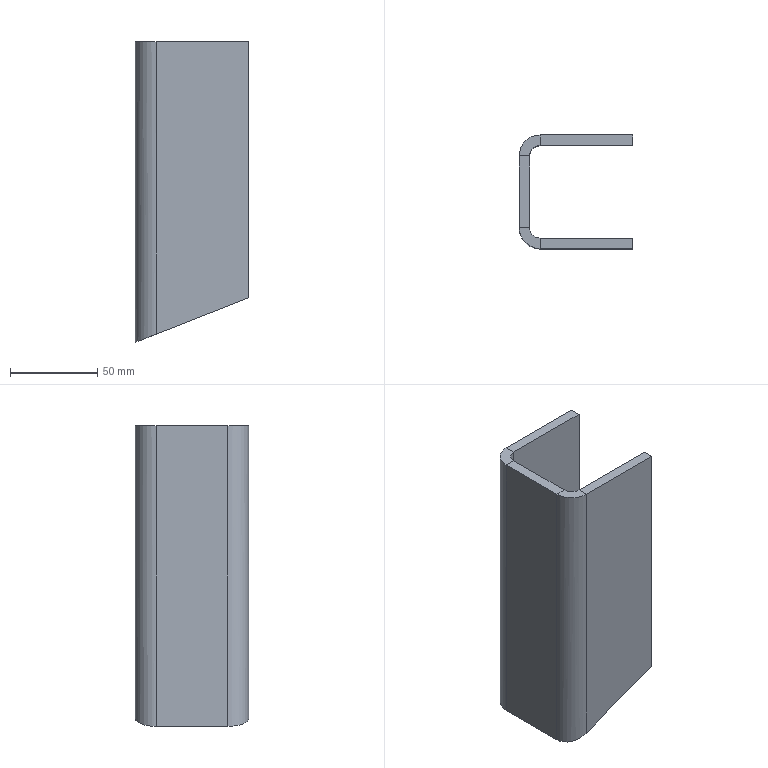Part | STEP file | 10-Bent plate | 1 solid | 18 faces | box 65 x 65 x 172 mm | volume 170584 mm3 | plane 14 | cylinder 4 | commonest cylinder face diameters 12 x2 24 x2
STEP:
#1=CARTESIAN_POINT('',(0.,0.,0.));
#2=DIRECTION('',(0.,0.,1.));
#3=DIRECTION('',(1.,0.,0.));
#4=AXIS2_PLACEMENT_3D('',#1,#2,#3);
#5=CARTESIAN_POINT('',(-53.,0.,172.));
#6=VERTEX_POINT('',#5);
#7=CARTESIAN_POINT('',(-53.,-6.,172.));
#8=VERTEX_POINT('',#7);
#9=CARTESIAN_POINT('',(-53.,0.,172.));
#10=DIRECTION('',(0.,-1.,0.));
#11=VECTOR('',#10,1.);
#12=LINE('',#9,#11);
#13=CARTESIAN_POINT('',(-53.,0.,172.));
#14=DIRECTION('',(0.,0.,1.));
#15=DIRECTION('',(1.,0.,0.));
#16=AXIS2_PLACEMENT_3D('',#13,#14,#15);
#17=PLANE('',#16);
#18=CARTESIAN_POINT('',(0.,0.));
#19=DIRECTION('',(0.,-1.));
#20=VECTOR('',#19,1.);
#21=LINE('',#18,#20);
#22=(GEOMETRIC_REPRESENTATION_CONTEXT(2)PARAMETRIC_REPRESENTATION_CONTEXT()REPRESENTATION_CONTEXT('',''));
#23=DEFINITIONAL_REPRESENTATION('',(#21),#22);
#24=PCURVE('',#17,#23);
#25=CARTESIAN_POINT('',(-59.,-12.,172.));
#26=DIRECTION('',(0.,0.,1.));
#27=DIRECTION('',(1.,0.,0.));
#28=AXIS2_PLACEMENT_3D('',#25,#26,#27);
#29=PLANE('',#28);
#30=CARTESIAN_POINT('',(6.,12.));
#31=DIRECTION('',(0.,-1.));
#32=VECTOR('',#31,1.);
#33=LINE('',#30,#32);
#34=(GEOMETRIC_REPRESENTATION_CONTEXT(2)PARAMETRIC_REPRESENTATION_CONTEXT()REPRESENTATION_CONTEXT('',''));
#35=DEFINITIONAL_REPRESENTATION('',(#33),#34);
#36=PCURVE('',#29,#35);
#37=SURFACE_CURVE('',#12,(#24,#36),.PCURVE_S1.);
#38=EDGE_CURVE('',#6,#8,#37,.T.);
#39=ORIENTED_EDGE('',*,*,#38,.F.);
#40=CARTESIAN_POINT('',(-65.,-12.,172.));
#41=VERTEX_POINT('',#40);
#42=CARTESIAN_POINT('',(-53.,-12.,172.));
#43=DIRECTION('',(0.,0.,1.));
#44=DIRECTION('',(-1.,0.,0.));
#45=AXIS2_PLACEMENT_3D('',#42,#43,#44);
#46=CIRCLE('',#45,12.);
#47=CARTESIAN_POINT('',(0.,-12.));
#48=DIRECTION('',(-1.,0.));
#49=AXIS2_PLACEMENT_2D('',#47,#48);
#50=CIRCLE('',#49,12.);
#51=(GEOMETRIC_REPRESENTATION_CONTEXT(2)PARAMETRIC_REPRESENTATION_CONTEXT()REPRESENTATION_CONTEXT('',''));
#52=DEFINITIONAL_REPRESENTATION('',(#50),#51);
#53=PCURVE('',#17,#52);
#54=CARTESIAN_POINT('',(-53.,-12.,172.));
#55=DIRECTION('',(0.,0.,-1.));
#56=DIRECTION('',(-1.,0.,0.));
#57=AXIS2_PLACEMENT_3D('',#54,#55,#56);
#58=CYLINDRICAL_SURFACE('',#57,12.);
#59=CARTESIAN_POINT('',(6.283,0.));
#60=DIRECTION('',(-1.,0.));
#61=VECTOR('',#60,1.);
#62=LINE('',#59,#61);
#63=(GEOMETRIC_REPRESENTATION_CONTEXT(2)PARAMETRIC_REPRESENTATION_CONTEXT()REPRESENTATION_CONTEXT('',''));
#64=DEFINITIONAL_REPRESENTATION('',(#62),#63);
#65=PCURVE('',#58,#64);
#66=SURFACE_CURVE('',#46,(#53,#65),.PCURVE_S1.);
#67=EDGE_CURVE('',#6,#41,#66,.T.);
#68=ORIENTED_EDGE('',*,*,#67,.T.);
#69=CARTESIAN_POINT('',(-59.,-12.,172.));
#70=VERTEX_POINT('',#69);
#71=CARTESIAN_POINT('',(-59.,-12.,172.));
#72=DIRECTION('',(-1.,0.,0.));
#73=VECTOR('',#72,1.);
#74=LINE('',#71,#73);
#75=CARTESIAN_POINT('',(-6.,-12.));
#76=DIRECTION('',(-1.,0.));
#77=VECTOR('',#76,1.);
#78=LINE('',#75,#77);
#79=(GEOMETRIC_REPRESENTATION_CONTEXT(2)PARAMETRIC_REPRESENTATION_CONTEXT()REPRESENTATION_CONTEXT('',''));
#80=DEFINITIONAL_REPRESENTATION('',(#78),#79);
#81=PCURVE('',#17,#80);
#82=CARTESIAN_POINT('',(-53.,-59.,172.));
#83=DIRECTION('',(0.,0.,1.));
#84=DIRECTION('',(1.,0.,0.));
#85=AXIS2_PLACEMENT_3D('',#82,#83,#84);
#86=PLANE('',#85);
#87=CARTESIAN_POINT('',(-6.,47.));
#88=DIRECTION('',(-1.,0.));
#89=VECTOR('',#88,1.);
#90=LINE('',#87,#89);
#91=(GEOMETRIC_REPRESENTATION_CONTEXT(2)PARAMETRIC_REPRESENTATION_CONTEXT()REPRESENTATION_CONTEXT('',''));
#92=DEFINITIONAL_REPRESENTATION('',(#90),#91);
#93=PCURVE('',#86,#92);
#94=SURFACE_CURVE('',#74,(#81,#93),.PCURVE_S1.);
#95=EDGE_CURVE('',#70,#41,#94,.T.);
#96=ORIENTED_EDGE('',*,*,#95,.F.);
#97=CARTESIAN_POINT('',(-53.,-12.,172.));
#98=DIRECTION('',(0.,0.,1.));
#99=DIRECTION('',(1.,0.,0.));
#100=AXIS2_PLACEMENT_3D('',#97,#98,#99);
#101=CIRCLE('',#100,6.);
#102=CARTESIAN_POINT('',(0.,-12.));
#103=DIRECTION('',(1.,0.));
#104=AXIS2_PLACEMENT_2D('',#102,#103);
#105=CIRCLE('',#104,6.);
#106=(GEOMETRIC_REPRESENTATION_CONTEXT(2)PARAMETRIC_REPRESENTATION_CONTEXT()REPRESENTATION_CONTEXT('',''));
#107=DEFINITIONAL_REPRESENTATION('',(#105),#106);
#108=PCURVE('',#17,#107);
#109=CARTESIAN_POINT('',(-53.,-12.,172.));
#110=DIRECTION('',(0.,0.,-1.));
#111=DIRECTION('',(-1.,0.,0.));
#112=AXIS2_PLACEMENT_3D('',#109,#110,#111);
#113=CYLINDRICAL_SURFACE('',#112,6.);
#114=CARTESIAN_POINT('',(3.142,0.));
#115=DIRECTION('',(-1.,0.));
#116=VECTOR('',#115,1.);
#117=LINE('',#114,#116);
#118=(GEOMETRIC_REPRESENTATION_CONTEXT(2)PARAMETRIC_REPRESENTATION_CONTEXT()REPRESENTATION_CONTEXT('',''));
#119=DEFINITIONAL_REPRESENTATION('',(#117),#118);
#120=PCURVE('',#113,#119);
#121=SURFACE_CURVE('',#101,(#108,#120),.PCURVE_S1.);
#122=EDGE_CURVE('',#8,#70,#121,.T.);
#123=ORIENTED_EDGE('',*,*,#122,.F.);
#124=EDGE_LOOP('',(#39,#68,#96,#123));
#125=FACE_BOUND('',#124,.T.);
#126=ADVANCED_FACE('',(#125),#17,.T.);
#127=CARTESIAN_POINT('',(0.,0.,172.));
#128=VERTEX_POINT('',#127);
#129=CARTESIAN_POINT('',(0.,0.,172.));
#130=DIRECTION('',(-1.,0.,0.));
#131=VECTOR('',#130,1.);
#132=LINE('',#129,#131);
#133=CARTESIAN_POINT('',(59.,12.));
#134=DIRECTION('',(-1.,0.));
#135=VECTOR('',#134,1.);
#136=LINE('',#133,#135);
#137=(GEOMETRIC_REPRESENTATION_CONTEXT(2)PARAMETRIC_REPRESENTATION_CONTEXT()REPRESENTATION_CONTEXT('',''));
#138=DEFINITIONAL_REPRESENTATION('',(#136),#137);
#139=PCURVE('',#29,#138);
#140=CARTESIAN_POINT('',(0.,0.,172.));
#141=DIRECTION('',(0.,-1.,0.));
#142=DIRECTION('',(1.,0.,0.));
#143=AXIS2_PLACEMENT_3D('',#140,#141,#142);
#144=PLANE('',#143);
#145=CARTESIAN_POINT('',(0.,0.));
#146=DIRECTION('',(-1.,0.));
#147=VECTOR('',#146,1.);
#148=LINE('',#145,#147);
#149=(GEOMETRIC_REPRESENTATION_CONTEXT(2)PARAMETRIC_REPRESENTATION_CONTEXT()REPRESENTATION_CONTEXT('',''));
#150=DEFINITIONAL_REPRESENTATION('',(#148),#149);
#151=PCURVE('',#144,#150);
#152=SURFACE_CURVE('',#132,(#139,#151),.PCURVE_S1.);
#153=EDGE_CURVE('',#128,#6,#152,.T.);
#154=ORIENTED_EDGE('',*,*,#153,.T.);
#155=ORIENTED_EDGE('',*,*,#38,.T.);
#156=CARTESIAN_POINT('',(0.,-6.,172.));
#157=VERTEX_POINT('',#156);
#158=CARTESIAN_POINT('',(0.,-6.,172.));
#159=DIRECTION('',(-1.,0.,0.));
#160=VECTOR('',#159,1.);
#161=LINE('',#158,#160);
#162=CARTESIAN_POINT('',(59.,6.));
#163=DIRECTION('',(-1.,0.));
#164=VECTOR('',#163,1.);
#165=LINE('',#162,#164);
#166=(GEOMETRIC_REPRESENTATION_CONTEXT(2)PARAMETRIC_REPRESENTATION_CONTEXT()REPRESENTATION_CONTEXT('',''));
#167=DEFINITIONAL_REPRESENTATION('',(#165),#166);
#168=PCURVE('',#29,#167);
#169=CARTESIAN_POINT('',(0.,-6.,172.));
#170=DIRECTION('',(0.,-1.,0.));
#171=DIRECTION('',(1.,0.,0.));
#172=AXIS2_PLACEMENT_3D('',#169,#170,#171);
#173=PLANE('',#172);
#174=CARTESIAN_POINT('',(0.,0.));
#175=DIRECTION('',(-1.,0.));
#176=VECTOR('',#175,1.);
#177=LINE('',#174,#176);
#178=(GEOMETRIC_REPRESENTATION_CONTEXT(2)PARAMETRIC_REPRESENTATION_CONTEXT()REPRESENTATION_CONTEXT('',''));
#179=DEFINITIONAL_REPRESENTATION('',(#177),#178);
#180=PCURVE('',#173,#179);
#181=SURFACE_CURVE('',#161,(#168,#180),.PCURVE_S1.);
#182=EDGE_CURVE('',#157,#8,#181,.T.);
#183=ORIENTED_EDGE('',*,*,#182,.F.);
#184=CARTESIAN_POINT('',(0.,0.,172.));
#185=DIRECTION('',(0.,-1.,0.));
#186=VECTOR('',#185,1.);
#187=LINE('',#184,#186);
#188=CARTESIAN_POINT('',(59.,12.));
#189=DIRECTION('',(0.,-1.));
#190=VECTOR('',#189,1.);
#191=LINE('',#188,#190);
#192=(GEOMETRIC_REPRESENTATION_CONTEXT(2)PARAMETRIC_REPRESENTATION_CONTEXT()REPRESENTATION_CONTEXT('',''));
#193=DEFINITIONAL_REPRESENTATION('',(#191),#192);
#194=PCURVE('',#29,#193);
#195=CARTESIAN_POINT('',(0.,0.,172.));
#196=DIRECTION('',(1.,0.,0.));
#197=DIRECTION('',(0.,1.,0.));
#198=AXIS2_PLACEMENT_3D('',#195,#196,#197);
#199=PLANE('',#198);
#200=CARTESIAN_POINT('',(0.,0.));
#201=DIRECTION('',(-1.,0.));
#202=VECTOR('',#201,1.);
#203=LINE('',#200,#202);
#204=(GEOMETRIC_REPRESENTATION_CONTEXT(2)PARAMETRIC_REPRESENTATION_CONTEXT()REPRESENTATION_CONTEXT('',''));
#205=DEFINITIONAL_REPRESENTATION('',(#203),#204);
#206=PCURVE('',#199,#205);
#207=SURFACE_CURVE('',#187,(#194,#206),.PCURVE_S1.);
#208=EDGE_CURVE('',#128,#157,#207,.T.);
#209=ORIENTED_EDGE('',*,*,#208,.F.);
#210=EDGE_LOOP('',(#154,#155,#183,#209));
#211=FACE_BOUND('',#210,.T.);
#212=ADVANCED_FACE('',(#211),#29,.T.);
#213=CARTESIAN_POINT('',(-65.,-53.,172.));
#214=VERTEX_POINT('',#213);
#215=CARTESIAN_POINT('',(-59.,-53.,172.));
#216=VERTEX_POINT('',#215);
#217=CARTESIAN_POINT('',(-65.,-53.,172.));
#218=DIRECTION('',(1.,0.,0.));
#219=VECTOR('',#218,1.);
#220=LINE('',#217,#219);
#221=CARTESIAN_POINT('',(-65.,-53.,172.));
#222=DIRECTION('',(0.,0.,1.));
#223=DIRECTION('',(1.,0.,0.));
#224=AXIS2_PLACEMENT_3D('',#221,#222,#223);
#225=PLANE('',#224);
#226=CARTESIAN_POINT('',(0.,0.));
#227=DIRECTION('',(1.,0.));
#228=VECTOR('',#227,1.);
#229=LINE('',#226,#228);
#230=(GEOMETRIC_REPRESENTATION_CONTEXT(2)PARAMETRIC_REPRESENTATION_CONTEXT()REPRESENTATION_CONTEXT('',''));
#231=DEFINITIONAL_REPRESENTATION('',(#229),#230);
#232=PCURVE('',#225,#231);
#233=CARTESIAN_POINT('',(-12.,6.));
#234=DIRECTION('',(1.,0.));
#235=VECTOR('',#234,1.);
#236=LINE('',#233,#235);
#237=(GEOMETRIC_REPRESENTATION_CONTEXT(2)PARAMETRIC_REPRESENTATION_CONTEXT()REPRESENTATION_CONTEXT('',''));
#238=DEFINITIONAL_REPRESENTATION('',(#236),#237);
#239=PCURVE('',#86,#238);
#240=SURFACE_CURVE('',#220,(#232,#239),.PCURVE_S1.);
#241=EDGE_CURVE('',#214,#216,#240,.T.);
#242=ORIENTED_EDGE('',*,*,#241,.F.);
#243=CARTESIAN_POINT('',(-53.,-65.,172.));
#244=VERTEX_POINT('',#243);
#245=CARTESIAN_POINT('',(-53.,-53.,172.));
#246=DIRECTION('',(0.,0.,1.));
#247=DIRECTION('',(-1.,0.,0.));
#248=AXIS2_PLACEMENT_3D('',#245,#246,#247);
#249=CIRCLE('',#248,12.);
#250=CARTESIAN_POINT('',(12.,0.));
#251=DIRECTION('',(-1.,0.));
#252=AXIS2_PLACEMENT_2D('',#250,#251);
#253=CIRCLE('',#252,12.);
#254=(GEOMETRIC_REPRESENTATION_CONTEXT(2)PARAMETRIC_REPRESENTATION_CONTEXT()REPRESENTATION_CONTEXT('',''));
#255=DEFINITIONAL_REPRESENTATION('',(#253),#254);
#256=PCURVE('',#225,#255);
#257=CARTESIAN_POINT('',(-53.,-53.,172.));
#258=DIRECTION('',(0.,0.,-1.));
#259=DIRECTION('',(-1.,0.,0.));
#260=AXIS2_PLACEMENT_3D('',#257,#258,#259);
#261=CYLINDRICAL_SURFACE('',#260,12.);
#262=CARTESIAN_POINT('',(6.283,0.));
#263=DIRECTION('',(-1.,0.));
#264=VECTOR('',#263,1.);
#265=LINE('',#262,#264);
#266=(GEOMETRIC_REPRESENTATION_CONTEXT(2)PARAMETRIC_REPRESENTATION_CONTEXT()REPRESENTATION_CONTEXT('',''));
#267=DEFINITIONAL_REPRESENTATION('',(#265),#266);
#268=PCURVE('',#261,#267);
#269=SURFACE_CURVE('',#249,(#256,#268),.PCURVE_S1.);
#270=EDGE_CURVE('',#214,#244,#269,.T.);
#271=ORIENTED_EDGE('',*,*,#270,.T.);
#272=CARTESIAN_POINT('',(-53.,-59.,172.));
#273=VERTEX_POINT('',#272);
#274=CARTESIAN_POINT('',(-53.,-59.,172.));
#275=DIRECTION('',(0.,-1.,0.));
#276=VECTOR('',#275,1.);
#277=LINE('',#274,#276);
#278=CARTESIAN_POINT('',(12.,-6.));
#279=DIRECTION('',(0.,-1.));
#280=VECTOR('',#279,1.);
#281=LINE('',#278,#280);
#282=(GEOMETRIC_REPRESENTATION_CONTEXT(2)PARAMETRIC_REPRESENTATION_CONTEXT()REPRESENTATION_CONTEXT('',''));
#283=DEFINITIONAL_REPRESENTATION('',(#281),#282);
#284=PCURVE('',#225,#283);
#285=CARTESIAN_POINT('',(-53.,-53.,172.));
#286=DIRECTION('',(0.,0.,1.));
#287=DIRECTION('',(1.,0.,0.));
#288=AXIS2_PLACEMENT_3D('',#285,#286,#287);
#289=PLANE('',#288);
#290=CARTESIAN_POINT('',(0.,-6.));
#291=DIRECTION('',(0.,-1.));
#292=VECTOR('',#291,1.);
#293=LINE('',#290,#292);
#294=(GEOMETRIC_REPRESENTATION_CONTEXT(2)PARAMETRIC_REPRESENTATION_CONTEXT()REPRESENTATION_CONTEXT('',''));
#295=DEFINITIONAL_REPRESENTATION('',(#293),#294);
#296=PCURVE('',#289,#295);
#297=SURFACE_CURVE('',#277,(#284,#296),.PCURVE_S1.);
#298=EDGE_CURVE('',#273,#244,#297,.T.);
#299=ORIENTED_EDGE('',*,*,#298,.F.);
#300=CARTESIAN_POINT('',(-53.,-53.,172.));
#301=DIRECTION('',(0.,0.,1.));
#302=DIRECTION('',(1.,0.,0.));
#303=AXIS2_PLACEMENT_3D('',#300,#301,#302);
#304=CIRCLE('',#303,6.);
#305=CARTESIAN_POINT('',(12.,0.));
#306=DIRECTION('',(1.,0.));
#307=AXIS2_PLACEMENT_2D('',#305,#306);
#308=CIRCLE('',#307,6.);
#309=(GEOMETRIC_REPRESENTATION_CONTEXT(2)PARAMETRIC_REPRESENTATION_CONTEXT()REPRESENTATION_CONTEXT('',''));
#310=DEFINITIONAL_REPRESENTATION('',(#308),#309);
#311=PCURVE('',#225,#310);
#312=CARTESIAN_POINT('',(-53.,-53.,172.));
#313=DIRECTION('',(0.,0.,-1.));
#314=DIRECTION('',(-1.,0.,0.));
#315=AXIS2_PLACEMENT_3D('',#312,#313,#314);
#316=CYLINDRICAL_SURFACE('',#315,6.);
#317=CARTESIAN_POINT('',(9.425,0.));
#318=DIRECTION('',(-1.,0.));
#319=VECTOR('',#318,1.);
#320=LINE('',#317,#319);
#321=(GEOMETRIC_REPRESENTATION_CONTEXT(2)PARAMETRIC_REPRESENTATION_CONTEXT()REPRESENTATION_CONTEXT('',''));
#322=DEFINITIONAL_REPRESENTATION('',(#320),#321);
#323=PCURVE('',#316,#322);
#324=SURFACE_CURVE('',#304,(#311,#323),.PCURVE_S1.);
#325=EDGE_CURVE('',#216,#273,#324,.T.);
#326=ORIENTED_EDGE('',*,*,#325,.F.);
#327=EDGE_LOOP('',(#242,#271,#299,#326));
#328=FACE_BOUND('',#327,.T.);
#329=ADVANCED_FACE('',(#328),#225,.T.);
#330=CARTESIAN_POINT('',(-65.,0.,172.));
#331=DIRECTION('',(0.,-1.,0.));
#332=VECTOR('',#331,1.);
#333=LINE('',#330,#332);
#334=CARTESIAN_POINT('',(-12.,59.));
#335=DIRECTION('',(0.,-1.));
#336=VECTOR('',#335,1.);
#337=LINE('',#334,#336);
#338=(GEOMETRIC_REPRESENTATION_CONTEXT(2)PARAMETRIC_REPRESENTATION_CONTEXT()REPRESENTATION_CONTEXT('',''));
#339=DEFINITIONAL_REPRESENTATION('',(#337),#338);
#340=PCURVE('',#86,#339);
#341=CARTESIAN_POINT('',(-65.,0.,172.));
#342=DIRECTION('',(1.,0.,0.));
#343=DIRECTION('',(0.,1.,0.));
#344=AXIS2_PLACEMENT_3D('',#341,#342,#343);
#345=PLANE('',#344);
#346=CARTESIAN_POINT('',(0.,0.));
#347=DIRECTION('',(-1.,0.));
#348=VECTOR('',#347,1.);
#349=LINE('',#346,#348);
#350=(GEOMETRIC_REPRESENTATION_CONTEXT(2)PARAMETRIC_REPRESENTATION_CONTEXT()REPRESENTATION_CONTEXT('',''));
#351=DEFINITIONAL_REPRESENTATION('',(#349),#350);
#352=PCURVE('',#345,#351);
#353=SURFACE_CURVE('',#333,(#340,#352),.PCURVE_S1.);
#354=EDGE_CURVE('',#41,#214,#353,.T.);
#355=ORIENTED_EDGE('',*,*,#354,.T.);
#356=ORIENTED_EDGE('',*,*,#241,.T.);
#357=CARTESIAN_POINT('',(-59.,0.,172.));
#358=DIRECTION('',(0.,-1.,0.));
#359=VECTOR('',#358,1.);
#360=LINE('',#357,#359);
#361=CARTESIAN_POINT('',(-6.,59.));
#362=DIRECTION('',(0.,-1.));
#363=VECTOR('',#362,1.);
#364=LINE('',#361,#363);
#365=(GEOMETRIC_REPRESENTATION_CONTEXT(2)PARAMETRIC_REPRESENTATION_CONTEXT()REPRESENTATION_CONTEXT('',''));
#366=DEFINITIONAL_REPRESENTATION('',(#364),#365);
#367=PCURVE('',#86,#366);
#368=CARTESIAN_POINT('',(-59.,0.,172.));
#369=DIRECTION('',(1.,0.,0.));
#370=DIRECTION('',(0.,1.,0.));
#371=AXIS2_PLACEMENT_3D('',#368,#369,#370);
#372=PLANE('',#371);
#373=CARTESIAN_POINT('',(0.,0.));
#374=DIRECTION('',(-1.,0.));
#375=VECTOR('',#374,1.);
#376=LINE('',#373,#375);
#377=(GEOMETRIC_REPRESENTATION_CONTEXT(2)PARAMETRIC_REPRESENTATION_CONTEXT()REPRESENTATION_CONTEXT('',''));
#378=DEFINITIONAL_REPRESENTATION('',(#376),#377);
#379=PCURVE('',#372,#378);
#380=SURFACE_CURVE('',#360,(#367,#379),.PCURVE_S1.);
#381=EDGE_CURVE('',#70,#216,#380,.T.);
#382=ORIENTED_EDGE('',*,*,#381,.F.);
#383=ORIENTED_EDGE('',*,*,#95,.T.);
#384=EDGE_LOOP('',(#355,#356,#382,#383));
#385=FACE_BOUND('',#384,.T.);
#386=ADVANCED_FACE('',(#385),#86,.T.);
#387=CARTESIAN_POINT('',(-53.,-65.,4.708));
#388=VERTEX_POINT('',#387);
#389=CARTESIAN_POINT('',(-53.,-65.,172.));
#390=DIRECTION('',(0.,0.,-1.));
#391=VECTOR('',#390,1.);
#392=LINE('',#389,#391);
#393=CARTESIAN_POINT('',(-65.,-65.,172.));
#394=DIRECTION('',(0.,1.,0.));
#395=DIRECTION('',(0.,0.,1.));
#396=AXIS2_PLACEMENT_3D('',#393,#394,#395);
#397=PLANE('',#396);
#398=CARTESIAN_POINT('',(0.,12.));
#399=DIRECTION('',(-1.,0.));
#400=VECTOR('',#399,1.);
#401=LINE('',#398,#400);
#402=(GEOMETRIC_REPRESENTATION_CONTEXT(2)PARAMETRIC_REPRESENTATION_CONTEXT()REPRESENTATION_CONTEXT('',''));
#403=DEFINITIONAL_REPRESENTATION('',(#401),#402);
#404=PCURVE('',#397,#403);
#405=CARTESIAN_POINT('',(4.712,0.));
#406=DIRECTION('',(0.,1.));
#407=VECTOR('',#406,1.);
#408=LINE('',#405,#407);
#409=(GEOMETRIC_REPRESENTATION_CONTEXT(2)PARAMETRIC_REPRESENTATION_CONTEXT()REPRESENTATION_CONTEXT('',''));
#410=DEFINITIONAL_REPRESENTATION('',(#408),#409);
#411=PCURVE('',#261,#410);
#412=SURFACE_CURVE('',#392,(#404,#411),.PCURVE_S1.);
#413=EDGE_CURVE('',#244,#388,#412,.T.);
#414=ORIENTED_EDGE('',*,*,#413,.T.);
#415=CARTESIAN_POINT('',(0.,-65.,25.5));
#416=VERTEX_POINT('',#415);
#417=CARTESIAN_POINT('',(-8.67,-65.,22.099));
#418=DIRECTION('',(0.9309,0.,0.3652));
#419=VECTOR('',#418,1.);
#420=LINE('',#417,#419);
#421=CARTESIAN_POINT('',(-149.901,56.33));
#422=DIRECTION('',(0.3652,0.9309));
#423=VECTOR('',#422,1.);
#424=LINE('',#421,#423);
#425=(GEOMETRIC_REPRESENTATION_CONTEXT(2)PARAMETRIC_REPRESENTATION_CONTEXT()REPRESENTATION_CONTEXT('',''));
#426=DEFINITIONAL_REPRESENTATION('',(#424),#425);
#427=PCURVE('',#397,#426);
#428=CARTESIAN_POINT('',(-8.67,-65.,22.099));
#429=DIRECTION('',(-0.3652,0.,0.9309));
#430=DIRECTION('',(0.9309,0.,0.3652));
#431=AXIS2_PLACEMENT_3D('',#428,#429,#430);
#432=PLANE('',#431);
#433=CARTESIAN_POINT('',(0.,0.));
#434=DIRECTION('',(1.,0.));
#435=VECTOR('',#434,1.);
#436=LINE('',#433,#435);
#437=(GEOMETRIC_REPRESENTATION_CONTEXT(2)PARAMETRIC_REPRESENTATION_CONTEXT()REPRESENTATION_CONTEXT('',''));
#438=DEFINITIONAL_REPRESENTATION('',(#436),#437);
#439=PCURVE('',#432,#438);
#440=SURFACE_CURVE('',#420,(#427,#439),.PCURVE_S1.);
#441=EDGE_CURVE('',#388,#416,#440,.T.);
#442=ORIENTED_EDGE('',*,*,#441,.T.);
#443=CARTESIAN_POINT('',(0.,-65.,172.));
#444=VERTEX_POINT('',#443);
#445=CARTESIAN_POINT('',(0.,-65.,172.));
#446=DIRECTION('',(0.,0.,-1.));
#447=VECTOR('',#446,1.);
#448=LINE('',#445,#447);
#449=CARTESIAN_POINT('',(0.,65.));
#450=DIRECTION('',(-1.,0.));
#451=VECTOR('',#450,1.);
#452=LINE('',#449,#451);
#453=(GEOMETRIC_REPRESENTATION_CONTEXT(2)PARAMETRIC_REPRESENTATION_CONTEXT()REPRESENTATION_CONTEXT('',''));
#454=DEFINITIONAL_REPRESENTATION('',(#452),#453);
#455=PCURVE('',#397,#454);
#456=CARTESIAN_POINT('',(0.,-59.,172.));
#457=DIRECTION('',(1.,0.,0.));
#458=DIRECTION('',(0.,0.,-1.));
#459=AXIS2_PLACEMENT_3D('',#456,#457,#458);
#460=PLANE('',#459);
#461=CARTESIAN_POINT('',(0.,-6.));
#462=DIRECTION('',(1.,0.));
#463=VECTOR('',#462,1.);
#464=LINE('',#461,#463);
#465=(GEOMETRIC_REPRESENTATION_CONTEXT(2)PARAMETRIC_REPRESENTATION_CONTEXT()REPRESENTATION_CONTEXT('',''));
#466=DEFINITIONAL_REPRESENTATION('',(#464),#465);
#467=PCURVE('',#460,#466);
#468=SURFACE_CURVE('',#448,(#455,#467),.PCURVE_S1.);
#469=EDGE_CURVE('',#444,#416,#468,.T.);
#470=ORIENTED_EDGE('',*,*,#469,.F.);
#471=CARTESIAN_POINT('',(-65.,-65.,172.));
#472=DIRECTION('',(1.,0.,0.));
#473=VECTOR('',#472,1.);
#474=LINE('',#471,#473);
#475=CARTESIAN_POINT('',(0.,0.));
#476=DIRECTION('',(0.,1.));
#477=VECTOR('',#476,1.);
#478=LINE('',#475,#477);
#479=(GEOMETRIC_REPRESENTATION_CONTEXT(2)PARAMETRIC_REPRESENTATION_CONTEXT()REPRESENTATION_CONTEXT('',''));
#480=DEFINITIONAL_REPRESENTATION('',(#478),#479);
#481=PCURVE('',#397,#480);
#482=CARTESIAN_POINT('',(-12.,-12.));
#483=DIRECTION('',(1.,0.));
#484=VECTOR('',#483,1.);
#485=LINE('',#482,#484);
#486=(GEOMETRIC_REPRESENTATION_CONTEXT(2)PARAMETRIC_REPRESENTATION_CONTEXT()REPRESENTATION_CONTEXT('',''));
#487=DEFINITIONAL_REPRESENTATION('',(#485),#486);
#488=PCURVE('',#289,#487);
#489=SURFACE_CURVE('',#474,(#481,#488),.PCURVE_S1.);
#490=EDGE_CURVE('',#244,#444,#489,.T.);
#491=ORIENTED_EDGE('',*,*,#490,.F.);
#492=EDGE_LOOP('',(#414,#442,#470,#491));
#493=FACE_BOUND('',#492,.T.);
#494=ADVANCED_FACE('',(#493),#397,.F.);
#495=CARTESIAN_POINT('',(0.,-59.,25.5));
#496=VERTEX_POINT('',#495);
#497=CARTESIAN_POINT('',(0.,-65.,25.5));
#498=DIRECTION('',(0.,1.,0.));
#499=VECTOR('',#498,1.);
#500=LINE('',#497,#499);
#501=CARTESIAN_POINT('',(146.5,-6.));
#502=DIRECTION('',(0.,1.));
#503=VECTOR('',#502,1.);
#504=LINE('',#501,#503);
#505=(GEOMETRIC_REPRESENTATION_CONTEXT(2)PARAMETRIC_REPRESENTATION_CONTEXT()REPRESENTATION_CONTEXT('',''));
#506=DEFINITIONAL_REPRESENTATION('',(#504),#505);
#507=PCURVE('',#460,#506);
#508=CARTESIAN_POINT('',(9.313,0.));
#509=DIRECTION('',(0.,1.));
#510=VECTOR('',#509,1.);
#511=LINE('',#508,#510);
#512=(GEOMETRIC_REPRESENTATION_CONTEXT(2)PARAMETRIC_REPRESENTATION_CONTEXT()REPRESENTATION_CONTEXT('',''));
#513=DEFINITIONAL_REPRESENTATION('',(#511),#512);
#514=PCURVE('',#432,#513);
#515=SURFACE_CURVE('',#500,(#507,#514),.PCURVE_S1.);
#516=EDGE_CURVE('',#416,#496,#515,.T.);
#517=ORIENTED_EDGE('',*,*,#516,.T.);
#518=CARTESIAN_POINT('',(0.,-59.,172.));
#519=VERTEX_POINT('',#518);
#520=CARTESIAN_POINT('',(0.,-59.,172.));
#521=DIRECTION('',(0.,0.,-1.));
#522=VECTOR('',#521,1.);
#523=LINE('',#520,#522);
#524=CARTESIAN_POINT('',(0.,0.));
#525=DIRECTION('',(1.,0.));
#526=VECTOR('',#525,1.);
#527=LINE('',#524,#526);
#528=(GEOMETRIC_REPRESENTATION_CONTEXT(2)PARAMETRIC_REPRESENTATION_CONTEXT()REPRESENTATION_CONTEXT('',''));
#529=DEFINITIONAL_REPRESENTATION('',(#527),#528);
#530=PCURVE('',#460,#529);
#531=CARTESIAN_POINT('',(-65.,-59.,172.));
#532=DIRECTION('',(0.,1.,0.));
#533=DIRECTION('',(0.,0.,1.));
#534=AXIS2_PLACEMENT_3D('',#531,#532,#533);
#535=PLANE('',#534);
#536=CARTESIAN_POINT('',(0.,65.));
#537=DIRECTION('',(-1.,0.));
#538=VECTOR('',#537,1.);
#539=LINE('',#536,#538);
#540=(GEOMETRIC_REPRESENTATION_CONTEXT(2)PARAMETRIC_REPRESENTATION_CONTEXT()REPRESENTATION_CONTEXT('',''));
#541=DEFINITIONAL_REPRESENTATION('',(#539),#540);
#542=PCURVE('',#535,#541);
#543=SURFACE_CURVE('',#523,(#530,#542),.PCURVE_S1.);
#544=EDGE_CURVE('',#519,#496,#543,.T.);
#545=ORIENTED_EDGE('',*,*,#544,.F.);
#546=CARTESIAN_POINT('',(0.,-59.,172.));
#547=DIRECTION('',(0.,-1.,0.));
#548=VECTOR('',#547,1.);
#549=LINE('',#546,#548);
#550=CARTESIAN_POINT('',(0.,0.));
#551=DIRECTION('',(0.,-1.));
#552=VECTOR('',#551,1.);
#553=LINE('',#550,#552);
#554=(GEOMETRIC_REPRESENTATION_CONTEXT(2)PARAMETRIC_REPRESENTATION_CONTEXT()REPRESENTATION_CONTEXT('',''));
#555=DEFINITIONAL_REPRESENTATION('',(#553),#554);
#556=PCURVE('',#460,#555);
#557=CARTESIAN_POINT('',(53.,-6.));
#558=DIRECTION('',(0.,-1.));
#559=VECTOR('',#558,1.);
#560=LINE('',#557,#559);
#561=(GEOMETRIC_REPRESENTATION_CONTEXT(2)PARAMETRIC_REPRESENTATION_CONTEXT()REPRESENTATION_CONTEXT('',''));
#562=DEFINITIONAL_REPRESENTATION('',(#560),#561);
#563=PCURVE('',#289,#562);
#564=SURFACE_CURVE('',#549,(#556,#563),.PCURVE_S1.);
#565=EDGE_CURVE('',#519,#444,#564,.T.);
#566=ORIENTED_EDGE('',*,*,#565,.T.);
#567=ORIENTED_EDGE('',*,*,#469,.T.);
#568=EDGE_LOOP('',(#517,#545,#566,#567));
#569=FACE_BOUND('',#568,.T.);
#570=ADVANCED_FACE('',(#569),#460,.T.);
#571=CARTESIAN_POINT('',(-53.,-59.,4.708));
#572=VERTEX_POINT('',#571);
#573=CARTESIAN_POINT('',(-6.523,-59.,22.941));
#574=DIRECTION('',(0.9309,0.,0.3652));
#575=VECTOR('',#574,1.);
#576=LINE('',#573,#575);
#577=CARTESIAN_POINT('',(-149.059,58.477));
#578=DIRECTION('',(0.3652,0.9309));
#579=VECTOR('',#578,1.);
#580=LINE('',#577,#579);
#581=(GEOMETRIC_REPRESENTATION_CONTEXT(2)PARAMETRIC_REPRESENTATION_CONTEXT()REPRESENTATION_CONTEXT('',''));
#582=DEFINITIONAL_REPRESENTATION('',(#580),#581);
#583=PCURVE('',#535,#582);
#584=CARTESIAN_POINT('',(2.306,6.));
#585=DIRECTION('',(1.,0.));
#586=VECTOR('',#585,1.);
#587=LINE('',#584,#586);
#588=(GEOMETRIC_REPRESENTATION_CONTEXT(2)PARAMETRIC_REPRESENTATION_CONTEXT()REPRESENTATION_CONTEXT('',''));
#589=DEFINITIONAL_REPRESENTATION('',(#587),#588);
#590=PCURVE('',#432,#589);
#591=SURFACE_CURVE('',#576,(#583,#590),.PCURVE_S1.);
#592=EDGE_CURVE('',#572,#496,#591,.T.);
#593=ORIENTED_EDGE('',*,*,#592,.F.);
#594=CARTESIAN_POINT('',(-53.,-59.,172.));
#595=DIRECTION('',(0.,0.,-1.));
#596=VECTOR('',#595,1.);
#597=LINE('',#594,#596);
#598=CARTESIAN_POINT('',(0.,12.));
#599=DIRECTION('',(-1.,0.));
#600=VECTOR('',#599,1.);
#601=LINE('',#598,#600);
#602=(GEOMETRIC_REPRESENTATION_CONTEXT(2)PARAMETRIC_REPRESENTATION_CONTEXT()REPRESENTATION_CONTEXT('',''));
#603=DEFINITIONAL_REPRESENTATION('',(#601),#602);
#604=PCURVE('',#535,#603);
#605=CARTESIAN_POINT('',(4.712,0.));
#606=DIRECTION('',(0.,1.));
#607=VECTOR('',#606,1.);
#608=LINE('',#605,#607);
#609=(GEOMETRIC_REPRESENTATION_CONTEXT(2)PARAMETRIC_REPRESENTATION_CONTEXT()REPRESENTATION_CONTEXT('',''));
#610=DEFINITIONAL_REPRESENTATION('',(#608),#609);
#611=PCURVE('',#316,#610);
#612=SURFACE_CURVE('',#597,(#604,#611),.PCURVE_S1.);
#613=EDGE_CURVE('',#273,#572,#612,.T.);
#614=ORIENTED_EDGE('',*,*,#613,.F.);
#615=CARTESIAN_POINT('',(-65.,-59.,172.));
#616=DIRECTION('',(1.,0.,0.));
#617=VECTOR('',#616,1.);
#618=LINE('',#615,#617);
#619=CARTESIAN_POINT('',(0.,0.));
#620=DIRECTION('',(0.,1.));
#621=VECTOR('',#620,1.);
#622=LINE('',#619,#621);
#623=(GEOMETRIC_REPRESENTATION_CONTEXT(2)PARAMETRIC_REPRESENTATION_CONTEXT()REPRESENTATION_CONTEXT('',''));
#624=DEFINITIONAL_REPRESENTATION('',(#622),#623);
#625=PCURVE('',#535,#624);
#626=CARTESIAN_POINT('',(-12.,-6.));
#627=DIRECTION('',(1.,0.));
#628=VECTOR('',#627,1.);
#629=LINE('',#626,#628);
#630=(GEOMETRIC_REPRESENTATION_CONTEXT(2)PARAMETRIC_REPRESENTATION_CONTEXT()REPRESENTATION_CONTEXT('',''));
#631=DEFINITIONAL_REPRESENTATION('',(#629),#630);
#632=PCURVE('',#289,#631);
#633=SURFACE_CURVE('',#618,(#625,#632),.PCURVE_S1.);
#634=EDGE_CURVE('',#273,#519,#633,.T.);
#635=ORIENTED_EDGE('',*,*,#634,.T.);
#636=ORIENTED_EDGE('',*,*,#544,.T.);
#637=EDGE_LOOP('',(#593,#614,#635,#636));
#638=FACE_BOUND('',#637,.T.);
#639=ADVANCED_FACE('',(#638),#535,.T.);
#640=ORIENTED_EDGE('',*,*,#613,.F.);
#641=ORIENTED_EDGE('',*,*,#325,.F.);
#642=CARTESIAN_POINT('',(-59.,-53.,2.354));
#643=VERTEX_POINT('',#642);
#644=CARTESIAN_POINT('',(-59.,-53.,172.));
#645=DIRECTION('',(0.,0.,-1.));
#646=VECTOR('',#645,1.);
#647=LINE('',#644,#646);
#648=CARTESIAN_POINT('',(6.283,0.));
#649=DIRECTION('',(0.,1.));
#650=VECTOR('',#649,1.);
#651=LINE('',#648,#650);
#652=(GEOMETRIC_REPRESENTATION_CONTEXT(2)PARAMETRIC_REPRESENTATION_CONTEXT()REPRESENTATION_CONTEXT('',''));
#653=DEFINITIONAL_REPRESENTATION('',(#651),#652);
#654=PCURVE('',#316,#653);
#655=CARTESIAN_POINT('',(-53.,0.));
#656=DIRECTION('',(0.,-1.));
#657=VECTOR('',#656,1.);
#658=LINE('',#655,#657);
#659=(GEOMETRIC_REPRESENTATION_CONTEXT(2)PARAMETRIC_REPRESENTATION_CONTEXT()REPRESENTATION_CONTEXT('',''));
#660=DEFINITIONAL_REPRESENTATION('',(#658),#659);
#661=PCURVE('',#372,#660);
#662=SURFACE_CURVE('',#647,(#654,#661),.PCURVE_S1.);
#663=EDGE_CURVE('',#216,#643,#662,.T.);
#664=ORIENTED_EDGE('',*,*,#663,.T.);
#665=CARTESIAN_POINT('',(-59.,-53.,2.354));
#666=CARTESIAN_POINT('',(-59.,-56.515,2.354));
#667=CARTESIAN_POINT('',(-56.515,-59.,3.329));
#668=CARTESIAN_POINT('',(-53.,-59.,4.708));
#669=(BOUNDED_CURVE()B_SPLINE_CURVE(3,(#665,#666,#667,#668),.UNSPECIFIED.,.F.,.F.)B_SPLINE_CURVE_WITH_KNOTS((4,4),(0.,1.571),.PIECEWISE_BEZIER_KNOTS.)CURVE()GEOMETRIC_REPRESENTATION_ITEM()RATIONAL_B_SPLINE_CURVE((1.,0.8047,0.8047,1.))REPRESENTATION_ITEM(''));
#670=CARTESIAN_POINT('',(6.283,169.646));
#671=CARTESIAN_POINT('',(6.262,169.646));
#672=CARTESIAN_POINT('',(6.218,169.643));
#673=CARTESIAN_POINT('',(6.152,169.628));
#674=CARTESIAN_POINT('',(6.083,169.601));
#675=CARTESIAN_POINT('',(6.013,169.563));
#676=CARTESIAN_POINT('',(5.942,169.513));
#677=CARTESIAN_POINT('',(5.87,169.45));
#678=CARTESIAN_POINT('',(5.797,169.375));
#679=CARTESIAN_POINT('',(5.723,169.288));
#680=CARTESIAN_POINT('',(5.648,169.189));
#681=CARTESIAN_POINT('',(5.573,169.079));
#682=CARTESIAN_POINT('',(5.498,168.958));
#683=CARTESIAN_POINT('',(5.422,168.828));
#684=CARTESIAN_POINT('',(5.347,168.69));
#685=CARTESIAN_POINT('',(5.273,168.544));
#686=CARTESIAN_POINT('',(5.199,168.393));
#687=CARTESIAN_POINT('',(5.125,168.238));
#688=CARTESIAN_POINT('',(5.053,168.08));
#689=CARTESIAN_POINT('',(4.982,167.92));
#690=CARTESIAN_POINT('',(4.912,167.76));
#691=CARTESIAN_POINT('',(4.844,167.601));
#692=CARTESIAN_POINT('',(4.777,167.445));
#693=CARTESIAN_POINT('',(4.734,167.343));
#694=CARTESIAN_POINT('',(4.712,167.292));
#695=B_SPLINE_CURVE_WITH_KNOTS('',3,(#670,#671,#672,#673,#674,#675,#676,#677,#678,#679,#680,#681,#682,#683,#684,#685,#686,#687,#688,#689,#690,#691,#692,#693,#694),.UNSPECIFIED.,.F.,.F.,(4,1,1,1,1,1,1,1,1,1,1,1,1,1,1,1,1,1,1,1,1,1,4),(0.,0.0714,0.1428,0.2142,0.2856,0.357,0.4284,0.4998,0.5712,0.6426,0.714,0.7854,0.8568,0.9282,0.9996,1.071,1.142,1.214,1.285,1.357,1.428,1.499,1.571),.QUASI_UNIFORM_KNOTS.);
#696=(GEOMETRIC_REPRESENTATION_CONTEXT(2)PARAMETRIC_REPRESENTATION_CONTEXT()REPRESENTATION_CONTEXT('',''));
#697=DEFINITIONAL_REPRESENTATION('',(#695),#696);
#698=PCURVE('',#316,#697);
#699=CARTESIAN_POINT('',(-54.065,12.));
#700=CARTESIAN_POINT('',(-54.065,8.485));
#701=CARTESIAN_POINT('',(-51.395,6.));
#702=CARTESIAN_POINT('',(-47.62,6.));
#703=(BOUNDED_CURVE()B_SPLINE_CURVE(3,(#699,#700,#701,#702),.UNSPECIFIED.,.F.,.F.)B_SPLINE_CURVE_WITH_KNOTS((4,4),(0.,1.571),.PIECEWISE_BEZIER_KNOTS.)CURVE()GEOMETRIC_REPRESENTATION_ITEM()RATIONAL_B_SPLINE_CURVE((1.,0.8047,0.8047,1.))REPRESENTATION_ITEM(''));
#704=(GEOMETRIC_REPRESENTATION_CONTEXT(2)PARAMETRIC_REPRESENTATION_CONTEXT()REPRESENTATION_CONTEXT('',''));
#705=DEFINITIONAL_REPRESENTATION('',(#703),#704);
#706=PCURVE('',#432,#705);
#707=SURFACE_CURVE('',#669,(#698,#706),.PCURVE_S1.);
#708=EDGE_CURVE('',#643,#572,#707,.T.);
#709=ORIENTED_EDGE('',*,*,#708,.T.);
#710=EDGE_LOOP('',(#640,#641,#664,#709));
#711=FACE_BOUND('',#710,.F.);
#712=ADVANCED_FACE('',(#711),#316,.F.);
#713=CARTESIAN_POINT('',(-59.,-12.,2.354));
#714=VERTEX_POINT('',#713);
#715=CARTESIAN_POINT('',(-59.,0.,2.354));
#716=DIRECTION('',(0.,-1.,0.));
#717=VECTOR('',#716,1.);
#718=LINE('',#715,#717);
#719=CARTESIAN_POINT('',(0.,-169.646));
#720=DIRECTION('',(-1.,0.));
#721=VECTOR('',#720,1.);
#722=LINE('',#719,#721);
#723=(GEOMETRIC_REPRESENTATION_CONTEXT(2)PARAMETRIC_REPRESENTATION_CONTEXT()REPRESENTATION_CONTEXT('',''));
#724=DEFINITIONAL_REPRESENTATION('',(#722),#723);
#725=PCURVE('',#372,#724);
#726=CARTESIAN_POINT('',(-54.065,65.));
#727=DIRECTION('',(0.,-1.));
#728=VECTOR('',#727,1.);
#729=LINE('',#726,#728);
#730=(GEOMETRIC_REPRESENTATION_CONTEXT(2)PARAMETRIC_REPRESENTATION_CONTEXT()REPRESENTATION_CONTEXT('',''));
#731=DEFINITIONAL_REPRESENTATION('',(#729),#730);
#732=PCURVE('',#432,#731);
#733=SURFACE_CURVE('',#718,(#725,#732),.PCURVE_S1.);
#734=EDGE_CURVE('',#714,#643,#733,.T.);
#735=ORIENTED_EDGE('',*,*,#734,.F.);
#736=CARTESIAN_POINT('',(-59.,-12.,172.));
#737=DIRECTION('',(0.,0.,-1.));
#738=VECTOR('',#737,1.);
#739=LINE('',#736,#738);
#740=CARTESIAN_POINT('',(-12.,0.));
#741=DIRECTION('',(0.,-1.));
#742=VECTOR('',#741,1.);
#743=LINE('',#740,#742);
#744=(GEOMETRIC_REPRESENTATION_CONTEXT(2)PARAMETRIC_REPRESENTATION_CONTEXT()REPRESENTATION_CONTEXT('',''));
#745=DEFINITIONAL_REPRESENTATION('',(#743),#744);
#746=PCURVE('',#372,#745);
#747=CARTESIAN_POINT('',(0.,0.));
#748=DIRECTION('',(0.,1.));
#749=VECTOR('',#748,1.);
#750=LINE('',#747,#749);
#751=(GEOMETRIC_REPRESENTATION_CONTEXT(2)PARAMETRIC_REPRESENTATION_CONTEXT()REPRESENTATION_CONTEXT('',''));
#752=DEFINITIONAL_REPRESENTATION('',(#750),#751);
#753=PCURVE('',#113,#752);
#754=SURFACE_CURVE('',#739,(#746,#753),.PCURVE_S1.);
#755=EDGE_CURVE('',#70,#714,#754,.T.);
#756=ORIENTED_EDGE('',*,*,#755,.F.);
#757=ORIENTED_EDGE('',*,*,#381,.T.);
#758=ORIENTED_EDGE('',*,*,#663,.T.);
#759=EDGE_LOOP('',(#735,#756,#757,#758));
#760=FACE_BOUND('',#759,.T.);
#761=ADVANCED_FACE('',(#760),#372,.T.);
#762=ORIENTED_EDGE('',*,*,#755,.F.);
#763=ORIENTED_EDGE('',*,*,#122,.F.);
#764=CARTESIAN_POINT('',(-53.,-6.,4.708));
#765=VERTEX_POINT('',#764);
#766=CARTESIAN_POINT('',(-53.,-6.,172.));
#767=DIRECTION('',(0.,0.,-1.));
#768=VECTOR('',#767,1.);
#769=LINE('',#766,#768);
#770=CARTESIAN_POINT('',(1.571,0.));
#771=DIRECTION('',(0.,1.));
#772=VECTOR('',#771,1.);
#773=LINE('',#770,#772);
#774=(GEOMETRIC_REPRESENTATION_CONTEXT(2)PARAMETRIC_REPRESENTATION_CONTEXT()REPRESENTATION_CONTEXT('',''));
#775=DEFINITIONAL_REPRESENTATION('',(#773),#774);
#776=PCURVE('',#113,#775);
#777=CARTESIAN_POINT('',(-53.,0.));
#778=DIRECTION('',(0.,-1.));
#779=VECTOR('',#778,1.);
#780=LINE('',#777,#779);
#781=(GEOMETRIC_REPRESENTATION_CONTEXT(2)PARAMETRIC_REPRESENTATION_CONTEXT()REPRESENTATION_CONTEXT('',''));
#782=DEFINITIONAL_REPRESENTATION('',(#780),#781);
#783=PCURVE('',#173,#782);
#784=SURFACE_CURVE('',#769,(#776,#783),.PCURVE_S1.);
#785=EDGE_CURVE('',#8,#765,#784,.T.);
#786=ORIENTED_EDGE('',*,*,#785,.T.);
#787=CARTESIAN_POINT('',(-53.,-6.,4.708));
#788=CARTESIAN_POINT('',(-56.515,-6.,3.329));
#789=CARTESIAN_POINT('',(-59.,-8.485,2.354));
#790=CARTESIAN_POINT('',(-59.,-12.,2.354));
#791=(BOUNDED_CURVE()B_SPLINE_CURVE(3,(#787,#788,#789,#790),.UNSPECIFIED.,.F.,.F.)B_SPLINE_CURVE_WITH_KNOTS((4,4),(4.712,6.283),.PIECEWISE_BEZIER_KNOTS.)CURVE()GEOMETRIC_REPRESENTATION_ITEM()RATIONAL_B_SPLINE_CURVE((1.,0.8047,0.8047,1.))REPRESENTATION_ITEM(''));
#792=CARTESIAN_POINT('',(1.571,167.292));
#793=CARTESIAN_POINT('',(1.549,167.343));
#794=CARTESIAN_POINT('',(1.506,167.445));
#795=CARTESIAN_POINT('',(1.439,167.601));
#796=CARTESIAN_POINT('',(1.371,167.76));
#797=CARTESIAN_POINT('',(1.301,167.92));
#798=CARTESIAN_POINT('',(1.23,168.08));
#799=CARTESIAN_POINT('',(1.158,168.238));
#800=CARTESIAN_POINT('',(1.085,168.393));
#801=CARTESIAN_POINT('',(1.01,168.544));
#802=CARTESIAN_POINT('',(0.9358,168.69));
#803=CARTESIAN_POINT('',(0.8607,168.828));
#804=CARTESIAN_POINT('',(0.7854,168.958));
#805=CARTESIAN_POINT('',(0.7101,169.079));
#806=CARTESIAN_POINT('',(0.635,169.189));
#807=CARTESIAN_POINT('',(0.5603,169.288));
#808=CARTESIAN_POINT('',(0.4863,169.375));
#809=CARTESIAN_POINT('',(0.413,169.45));
#810=CARTESIAN_POINT('',(0.3408,169.513));
#811=CARTESIAN_POINT('',(0.2697,169.563));
#812=CARTESIAN_POINT('',(0.2,169.601));
#813=CARTESIAN_POINT('',(0.1316,169.628));
#814=CARTESIAN_POINT('',(0.06485,169.643));
#815=CARTESIAN_POINT('',(0.02143,169.646));
#816=CARTESIAN_POINT('',(0.,169.646));
#817=B_SPLINE_CURVE_WITH_KNOTS('',3,(#792,#793,#794,#795,#796,#797,#798,#799,#800,#801,#802,#803,#804,#805,#806,#807,#808,#809,#810,#811,#812,#813,#814,#815,#816),.UNSPECIFIED.,.F.,.F.,(4,1,1,1,1,1,1,1,1,1,1,1,1,1,1,1,1,1,1,1,1,1,4),(4.712,4.784,4.855,4.927,4.998,5.069,5.141,5.212,5.284,5.355,5.426,5.498,5.569,5.641,5.712,5.783,5.855,5.926,5.998,6.069,6.14,6.212,6.283),.QUASI_UNIFORM_KNOTS.);
#818=(GEOMETRIC_REPRESENTATION_CONTEXT(2)PARAMETRIC_REPRESENTATION_CONTEXT()REPRESENTATION_CONTEXT('',''));
#819=DEFINITIONAL_REPRESENTATION('',(#817),#818);
#820=PCURVE('',#113,#819);
#821=CARTESIAN_POINT('',(-47.62,59.));
#822=CARTESIAN_POINT('',(-51.395,59.));
#823=CARTESIAN_POINT('',(-54.065,56.515));
#824=CARTESIAN_POINT('',(-54.065,53.));
#825=(BOUNDED_CURVE()B_SPLINE_CURVE(3,(#821,#822,#823,#824),.UNSPECIFIED.,.F.,.F.)B_SPLINE_CURVE_WITH_KNOTS((4,4),(4.712,6.283),.PIECEWISE_BEZIER_KNOTS.)CURVE()GEOMETRIC_REPRESENTATION_ITEM()RATIONAL_B_SPLINE_CURVE((1.,0.8047,0.8047,1.))REPRESENTATION_ITEM(''));
#826=(GEOMETRIC_REPRESENTATION_CONTEXT(2)PARAMETRIC_REPRESENTATION_CONTEXT()REPRESENTATION_CONTEXT('',''));
#827=DEFINITIONAL_REPRESENTATION('',(#825),#826);
#828=PCURVE('',#432,#827);
#829=SURFACE_CURVE('',#791,(#820,#828),.PCURVE_S1.);
#830=EDGE_CURVE('',#765,#714,#829,.T.);
#831=ORIENTED_EDGE('',*,*,#830,.T.);
#832=EDGE_LOOP('',(#762,#763,#786,#831));
#833=FACE_BOUND('',#832,.F.);
#834=ADVANCED_FACE('',(#833),#113,.F.);
#835=CARTESIAN_POINT('',(0.,-6.,25.5));
#836=VERTEX_POINT('',#835);
#837=CARTESIAN_POINT('',(49.807,-6.,45.04));
#838=DIRECTION('',(-0.9309,0.,-0.3652));
#839=VECTOR('',#838,1.);
#840=LINE('',#837,#839);
#841=CARTESIAN_POINT('',(49.807,-126.96));
#842=DIRECTION('',(-0.9309,-0.3652));
#843=VECTOR('',#842,1.);
#844=LINE('',#841,#843);
#845=(GEOMETRIC_REPRESENTATION_CONTEXT(2)PARAMETRIC_REPRESENTATION_CONTEXT()REPRESENTATION_CONTEXT('',''));
#846=DEFINITIONAL_REPRESENTATION('',(#844),#845);
#847=PCURVE('',#173,#846);
#848=CARTESIAN_POINT('',(62.816,59.));
#849=DIRECTION('',(-1.,0.));
#850=VECTOR('',#849,1.);
#851=LINE('',#848,#850);
#852=(GEOMETRIC_REPRESENTATION_CONTEXT(2)PARAMETRIC_REPRESENTATION_CONTEXT()REPRESENTATION_CONTEXT('',''));
#853=DEFINITIONAL_REPRESENTATION('',(#851),#852);
#854=PCURVE('',#432,#853);
#855=SURFACE_CURVE('',#840,(#847,#854),.PCURVE_S1.);
#856=EDGE_CURVE('',#836,#765,#855,.T.);
#857=ORIENTED_EDGE('',*,*,#856,.F.);
#858=CARTESIAN_POINT('',(0.,-6.,172.));
#859=DIRECTION('',(0.,0.,-1.));
#860=VECTOR('',#859,1.);
#861=LINE('',#858,#860);
#862=CARTESIAN_POINT('',(0.,0.));
#863=DIRECTION('',(0.,-1.));
#864=VECTOR('',#863,1.);
#865=LINE('',#862,#864);
#866=(GEOMETRIC_REPRESENTATION_CONTEXT(2)PARAMETRIC_REPRESENTATION_CONTEXT()REPRESENTATION_CONTEXT('',''));
#867=DEFINITIONAL_REPRESENTATION('',(#865),#866);
#868=PCURVE('',#173,#867);
#869=CARTESIAN_POINT('',(-6.,0.));
#870=DIRECTION('',(0.,-1.));
#871=VECTOR('',#870,1.);
#872=LINE('',#869,#871);
#873=(GEOMETRIC_REPRESENTATION_CONTEXT(2)PARAMETRIC_REPRESENTATION_CONTEXT()REPRESENTATION_CONTEXT('',''));
#874=DEFINITIONAL_REPRESENTATION('',(#872),#873);
#875=PCURVE('',#199,#874);
#876=SURFACE_CURVE('',#861,(#868,#875),.PCURVE_S1.);
#877=EDGE_CURVE('',#157,#836,#876,.T.);
#878=ORIENTED_EDGE('',*,*,#877,.F.);
#879=ORIENTED_EDGE('',*,*,#182,.T.);
#880=ORIENTED_EDGE('',*,*,#785,.T.);
#881=EDGE_LOOP('',(#857,#878,#879,#880));
#882=FACE_BOUND('',#881,.T.);
#883=ADVANCED_FACE('',(#882),#173,.T.);
#884=CARTESIAN_POINT('',(0.,0.,25.5));
#885=VERTEX_POINT('',#884);
#886=CARTESIAN_POINT('',(0.,-65.,25.5));
#887=DIRECTION('',(0.,1.,0.));
#888=VECTOR('',#887,1.);
#889=LINE('',#886,#888);
#890=CARTESIAN_POINT('',(-65.,-146.5));
#891=DIRECTION('',(1.,0.));
#892=VECTOR('',#891,1.);
#893=LINE('',#890,#892);
#894=(GEOMETRIC_REPRESENTATION_CONTEXT(2)PARAMETRIC_REPRESENTATION_CONTEXT()REPRESENTATION_CONTEXT('',''));
#895=DEFINITIONAL_REPRESENTATION('',(#893),#894);
#896=PCURVE('',#199,#895);
#897=CARTESIAN_POINT('',(9.313,0.));
#898=DIRECTION('',(0.,1.));
#899=VECTOR('',#898,1.);
#900=LINE('',#897,#899);
#901=(GEOMETRIC_REPRESENTATION_CONTEXT(2)PARAMETRIC_REPRESENTATION_CONTEXT()REPRESENTATION_CONTEXT('',''));
#902=DEFINITIONAL_REPRESENTATION('',(#900),#901);
#903=PCURVE('',#432,#902);
#904=SURFACE_CURVE('',#889,(#896,#903),.PCURVE_S1.);
#905=EDGE_CURVE('',#836,#885,#904,.T.);
#906=ORIENTED_EDGE('',*,*,#905,.T.);
#907=CARTESIAN_POINT('',(0.,0.,172.));
#908=DIRECTION('',(0.,0.,-1.));
#909=VECTOR('',#908,1.);
#910=LINE('',#907,#909);
#911=CARTESIAN_POINT('',(0.,0.));
#912=DIRECTION('',(0.,-1.));
#913=VECTOR('',#912,1.);
#914=LINE('',#911,#913);
#915=(GEOMETRIC_REPRESENTATION_CONTEXT(2)PARAMETRIC_REPRESENTATION_CONTEXT()REPRESENTATION_CONTEXT('',''));
#916=DEFINITIONAL_REPRESENTATION('',(#914),#915);
#917=PCURVE('',#199,#916);
#918=CARTESIAN_POINT('',(0.,0.));
#919=DIRECTION('',(0.,-1.));
#920=VECTOR('',#919,1.);
#921=LINE('',#918,#920);
#922=(GEOMETRIC_REPRESENTATION_CONTEXT(2)PARAMETRIC_REPRESENTATION_CONTEXT()REPRESENTATION_CONTEXT('',''));
#923=DEFINITIONAL_REPRESENTATION('',(#921),#922);
#924=PCURVE('',#144,#923);
#925=SURFACE_CURVE('',#910,(#917,#924),.PCURVE_S1.);
#926=EDGE_CURVE('',#128,#885,#925,.T.);
#927=ORIENTED_EDGE('',*,*,#926,.F.);
#928=ORIENTED_EDGE('',*,*,#208,.T.);
#929=ORIENTED_EDGE('',*,*,#877,.T.);
#930=EDGE_LOOP('',(#906,#927,#928,#929));
#931=FACE_BOUND('',#930,.T.);
#932=ADVANCED_FACE('',(#931),#199,.T.);
#933=ORIENTED_EDGE('',*,*,#926,.T.);
#934=CARTESIAN_POINT('',(-53.,0.,4.708));
#935=VERTEX_POINT('',#934);
#936=CARTESIAN_POINT('',(-8.67,0.,22.099));
#937=DIRECTION('',(0.9309,0.,0.3652));
#938=VECTOR('',#937,1.);
#939=LINE('',#936,#938);
#940=CARTESIAN_POINT('',(-8.67,-149.901));
#941=DIRECTION('',(0.9309,0.3652));
#942=VECTOR('',#941,1.);
#943=LINE('',#940,#942);
#944=(GEOMETRIC_REPRESENTATION_CONTEXT(2)PARAMETRIC_REPRESENTATION_CONTEXT()REPRESENTATION_CONTEXT('',''));
#945=DEFINITIONAL_REPRESENTATION('',(#943),#944);
#946=PCURVE('',#144,#945);
#947=CARTESIAN_POINT('',(0.,65.));
#948=DIRECTION('',(1.,0.));
#949=VECTOR('',#948,1.);
#950=LINE('',#947,#949);
#951=(GEOMETRIC_REPRESENTATION_CONTEXT(2)PARAMETRIC_REPRESENTATION_CONTEXT()REPRESENTATION_CONTEXT('',''));
#952=DEFINITIONAL_REPRESENTATION('',(#950),#951);
#953=PCURVE('',#432,#952);
#954=SURFACE_CURVE('',#939,(#946,#953),.PCURVE_S1.);
#955=EDGE_CURVE('',#935,#885,#954,.T.);
#956=ORIENTED_EDGE('',*,*,#955,.F.);
#957=CARTESIAN_POINT('',(-53.,0.,172.));
#958=DIRECTION('',(0.,0.,-1.));
#959=VECTOR('',#958,1.);
#960=LINE('',#957,#959);
#961=CARTESIAN_POINT('',(-53.,0.));
#962=DIRECTION('',(0.,-1.));
#963=VECTOR('',#962,1.);
#964=LINE('',#961,#963);
#965=(GEOMETRIC_REPRESENTATION_CONTEXT(2)PARAMETRIC_REPRESENTATION_CONTEXT()REPRESENTATION_CONTEXT('',''));
#966=DEFINITIONAL_REPRESENTATION('',(#964),#965);
#967=PCURVE('',#144,#966);
#968=CARTESIAN_POINT('',(1.571,0.));
#969=DIRECTION('',(0.,1.));
#970=VECTOR('',#969,1.);
#971=LINE('',#968,#970);
#972=(GEOMETRIC_REPRESENTATION_CONTEXT(2)PARAMETRIC_REPRESENTATION_CONTEXT()REPRESENTATION_CONTEXT('',''));
#973=DEFINITIONAL_REPRESENTATION('',(#971),#972);
#974=PCURVE('',#58,#973);
#975=SURFACE_CURVE('',#960,(#967,#974),.PCURVE_S1.);
#976=EDGE_CURVE('',#6,#935,#975,.T.);
#977=ORIENTED_EDGE('',*,*,#976,.F.);
#978=ORIENTED_EDGE('',*,*,#153,.F.);
#979=EDGE_LOOP('',(#933,#956,#977,#978));
#980=FACE_BOUND('',#979,.T.);
#981=ADVANCED_FACE('',(#980),#144,.F.);
#982=ORIENTED_EDGE('',*,*,#976,.T.);
#983=CARTESIAN_POINT('',(-65.,-12.,0.));
#984=VERTEX_POINT('',#983);
#985=CARTESIAN_POINT('',(-53.,0.,4.708));
#986=CARTESIAN_POINT('',(-60.029,0.,1.95));
#987=CARTESIAN_POINT('',(-65.,-4.971,0.));
#988=CARTESIAN_POINT('',(-65.,-12.,0.));
#989=(BOUNDED_CURVE()B_SPLINE_CURVE(3,(#985,#986,#987,#988),.UNSPECIFIED.,.F.,.F.)B_SPLINE_CURVE_WITH_KNOTS((4,4),(4.712,6.283),.PIECEWISE_BEZIER_KNOTS.)CURVE()GEOMETRIC_REPRESENTATION_ITEM()RATIONAL_B_SPLINE_CURVE((1.,0.8047,0.8047,1.))REPRESENTATION_ITEM(''));
#990=CARTESIAN_POINT('',(1.571,167.292));
#991=CARTESIAN_POINT('',(1.549,167.393));
#992=CARTESIAN_POINT('',(1.506,167.598));
#993=CARTESIAN_POINT('',(1.439,167.911));
#994=CARTESIAN_POINT('',(1.371,168.228));
#995=CARTESIAN_POINT('',(1.301,168.548));
#996=CARTESIAN_POINT('',(1.23,168.867));
#997=CARTESIAN_POINT('',(1.158,169.184));
#998=CARTESIAN_POINT('',(1.085,169.494));
#999=CARTESIAN_POINT('',(1.01,169.797));
#1000=CARTESIAN_POINT('',(0.9358,170.087));
#1001=CARTESIAN_POINT('',(0.8607,170.364));
#1002=CARTESIAN_POINT('',(0.7854,170.624));
#1003=CARTESIAN_POINT('',(0.7101,170.866));
#1004=CARTESIAN_POINT('',(0.635,171.086));
#1005=CARTESIAN_POINT('',(0.5603,171.284));
#1006=CARTESIAN_POINT('',(0.4863,171.458));
#1007=CARTESIAN_POINT('',(0.413,171.608));
#1008=CARTESIAN_POINT('',(0.3408,171.733));
#1009=CARTESIAN_POINT('',(0.2697,171.834));
#1010=CARTESIAN_POINT('',(0.2,171.91));
#1011=CARTESIAN_POINT('',(0.1316,171.963));
#1012=CARTESIAN_POINT('',(0.06485,171.994));
#1013=CARTESIAN_POINT('',(0.02143,172.));
#1014=CARTESIAN_POINT('',(0.,172.));
#1015=B_SPLINE_CURVE_WITH_KNOTS('',3,(#990,#991,#992,#993,#994,#995,#996,#997,#998,#999,#1000,#1001,#1002,#1003,#1004,#1005,#1006,#1007,#1008,#1009,#1010,#1011,#1012,#1013,#1014),.UNSPECIFIED.,.F.,.F.,(4,1,1,1,1,1,1,1,1,1,1,1,1,1,1,1,1,1,1,1,1,1,4),(4.712,4.784,4.855,4.927,4.998,5.069,5.141,5.212,5.284,5.355,5.426,5.498,5.569,5.641,5.712,5.783,5.855,5.926,5.998,6.069,6.14,6.212,6.283),.QUASI_UNIFORM_KNOTS.);
#1016=(GEOMETRIC_REPRESENTATION_CONTEXT(2)PARAMETRIC_REPRESENTATION_CONTEXT()REPRESENTATION_CONTEXT('',''));
#1017=DEFINITIONAL_REPRESENTATION('',(#1015),#1016);
#1018=PCURVE('',#58,#1017);
#1019=CARTESIAN_POINT('',(-47.62,65.));
#1020=CARTESIAN_POINT('',(-55.171,65.));
#1021=CARTESIAN_POINT('',(-60.51,60.029));
#1022=CARTESIAN_POINT('',(-60.51,53.));
#1023=(BOUNDED_CURVE()B_SPLINE_CURVE(3,(#1019,#1020,#1021,#1022),.UNSPECIFIED.,.F.,.F.)B_SPLINE_CURVE_WITH_KNOTS((4,4),(4.712,6.283),.PIECEWISE_BEZIER_KNOTS.)CURVE()GEOMETRIC_REPRESENTATION_ITEM()RATIONAL_B_SPLINE_CURVE((1.,0.8047,0.8047,1.))REPRESENTATION_ITEM(''));
#1024=(GEOMETRIC_REPRESENTATION_CONTEXT(2)PARAMETRIC_REPRESENTATION_CONTEXT()REPRESENTATION_CONTEXT('',''));
#1025=DEFINITIONAL_REPRESENTATION('',(#1023),#1024);
#1026=PCURVE('',#432,#1025);
#1027=SURFACE_CURVE('',#989,(#1018,#1026),.PCURVE_S1.);
#1028=EDGE_CURVE('',#935,#984,#1027,.T.);
#1029=ORIENTED_EDGE('',*,*,#1028,.T.);
#1030=CARTESIAN_POINT('',(-65.,-12.,172.));
#1031=DIRECTION('',(0.,0.,-1.));
#1032=VECTOR('',#1031,1.);
#1033=LINE('',#1030,#1032);
#1034=CARTESIAN_POINT('',(0.,0.));
#1035=DIRECTION('',(0.,1.));
#1036=VECTOR('',#1035,1.);
#1037=LINE('',#1034,#1036);
#1038=(GEOMETRIC_REPRESENTATION_CONTEXT(2)PARAMETRIC_REPRESENTATION_CONTEXT()REPRESENTATION_CONTEXT('',''));
#1039=DEFINITIONAL_REPRESENTATION('',(#1037),#1038);
#1040=PCURVE('',#58,#1039);
#1041=CARTESIAN_POINT('',(-12.,0.));
#1042=DIRECTION('',(0.,-1.));
#1043=VECTOR('',#1042,1.);
#1044=LINE('',#1041,#1043);
#1045=(GEOMETRIC_REPRESENTATION_CONTEXT(2)PARAMETRIC_REPRESENTATION_CONTEXT()REPRESENTATION_CONTEXT('',''));
#1046=DEFINITIONAL_REPRESENTATION('',(#1044),#1045);
#1047=PCURVE('',#345,#1046);
#1048=SURFACE_CURVE('',#1033,(#1040,#1047),.PCURVE_S1.);
#1049=EDGE_CURVE('',#41,#984,#1048,.T.);
#1050=ORIENTED_EDGE('',*,*,#1049,.F.);
#1051=ORIENTED_EDGE('',*,*,#67,.F.);
#1052=EDGE_LOOP('',(#982,#1029,#1050,#1051));
#1053=FACE_BOUND('',#1052,.T.);
#1054=ADVANCED_FACE('',(#1053),#58,.T.);
#1055=CARTESIAN_POINT('',(-65.,-53.,0.));
#1056=VERTEX_POINT('',#1055);
#1057=CARTESIAN_POINT('',(-65.,0.,0.));
#1058=DIRECTION('',(0.,-1.,0.));
#1059=VECTOR('',#1058,1.);
#1060=LINE('',#1057,#1059);
#1061=CARTESIAN_POINT('',(0.,-172.));
#1062=DIRECTION('',(-1.,0.));
#1063=VECTOR('',#1062,1.);
#1064=LINE('',#1061,#1063);
#1065=(GEOMETRIC_REPRESENTATION_CONTEXT(2)PARAMETRIC_REPRESENTATION_CONTEXT()REPRESENTATION_CONTEXT('',''));
#1066=DEFINITIONAL_REPRESENTATION('',(#1064),#1065);
#1067=PCURVE('',#345,#1066);
#1068=CARTESIAN_POINT('',(-60.51,65.));
#1069=DIRECTION('',(0.,-1.));
#1070=VECTOR('',#1069,1.);
#1071=LINE('',#1068,#1070);
#1072=(GEOMETRIC_REPRESENTATION_CONTEXT(2)PARAMETRIC_REPRESENTATION_CONTEXT()REPRESENTATION_CONTEXT('',''));
#1073=DEFINITIONAL_REPRESENTATION('',(#1071),#1072);
#1074=PCURVE('',#432,#1073);
#1075=SURFACE_CURVE('',#1060,(#1067,#1074),.PCURVE_S1.);
#1076=EDGE_CURVE('',#984,#1056,#1075,.T.);
#1077=ORIENTED_EDGE('',*,*,#1076,.T.);
#1078=CARTESIAN_POINT('',(-65.,-53.,172.));
#1079=DIRECTION('',(0.,0.,-1.));
#1080=VECTOR('',#1079,1.);
#1081=LINE('',#1078,#1080);
#1082=CARTESIAN_POINT('',(-53.,0.));
#1083=DIRECTION('',(0.,-1.));
#1084=VECTOR('',#1083,1.);
#1085=LINE('',#1082,#1084);
#1086=(GEOMETRIC_REPRESENTATION_CONTEXT(2)PARAMETRIC_REPRESENTATION_CONTEXT()REPRESENTATION_CONTEXT('',''));
#1087=DEFINITIONAL_REPRESENTATION('',(#1085),#1086);
#1088=PCURVE('',#345,#1087);
#1089=CARTESIAN_POINT('',(6.283,0.));
#1090=DIRECTION('',(0.,1.));
#1091=VECTOR('',#1090,1.);
#1092=LINE('',#1089,#1091);
#1093=(GEOMETRIC_REPRESENTATION_CONTEXT(2)PARAMETRIC_REPRESENTATION_CONTEXT()REPRESENTATION_CONTEXT('',''));
#1094=DEFINITIONAL_REPRESENTATION('',(#1092),#1093);
#1095=PCURVE('',#261,#1094);
#1096=SURFACE_CURVE('',#1081,(#1088,#1095),.PCURVE_S1.);
#1097=EDGE_CURVE('',#214,#1056,#1096,.T.);
#1098=ORIENTED_EDGE('',*,*,#1097,.F.);
#1099=ORIENTED_EDGE('',*,*,#354,.F.);
#1100=ORIENTED_EDGE('',*,*,#1049,.T.);
#1101=EDGE_LOOP('',(#1077,#1098,#1099,#1100));
#1102=FACE_BOUND('',#1101,.T.);
#1103=ADVANCED_FACE('',(#1102),#345,.F.);
#1104=ORIENTED_EDGE('',*,*,#1097,.T.);
#1105=CARTESIAN_POINT('',(-65.,-53.,0.));
#1106=CARTESIAN_POINT('',(-65.,-60.029,0.));
#1107=CARTESIAN_POINT('',(-60.029,-65.,1.95));
#1108=CARTESIAN_POINT('',(-53.,-65.,4.708));
#1109=(BOUNDED_CURVE()B_SPLINE_CURVE(3,(#1105,#1106,#1107,#1108),.UNSPECIFIED.,.F.,.F.)B_SPLINE_CURVE_WITH_KNOTS((4,4),(0.,1.571),.PIECEWISE_BEZIER_KNOTS.)CURVE()GEOMETRIC_REPRESENTATION_ITEM()RATIONAL_B_SPLINE_CURVE((1.,0.8047,0.8047,1.))REPRESENTATION_ITEM(''));
#1110=CARTESIAN_POINT('',(6.283,172.));
#1111=CARTESIAN_POINT('',(6.262,172.));
#1112=CARTESIAN_POINT('',(6.218,171.994));
#1113=CARTESIAN_POINT('',(6.152,171.963));
#1114=CARTESIAN_POINT('',(6.083,171.91));
#1115=CARTESIAN_POINT('',(6.013,171.834));
#1116=CARTESIAN_POINT('',(5.942,171.733));
#1117=CARTESIAN_POINT('',(5.87,171.608));
#1118=CARTESIAN_POINT('',(5.797,171.458));
#1119=CARTESIAN_POINT('',(5.723,171.284));
#1120=CARTESIAN_POINT('',(5.648,171.086));
#1121=CARTESIAN_POINT('',(5.573,170.866));
#1122=CARTESIAN_POINT('',(5.498,170.624));
#1123=CARTESIAN_POINT('',(5.422,170.364));
#1124=CARTESIAN_POINT('',(5.347,170.087));
#1125=CARTESIAN_POINT('',(5.273,169.797));
#1126=CARTESIAN_POINT('',(5.199,169.494));
#1127=CARTESIAN_POINT('',(5.125,169.184));
#1128=CARTESIAN_POINT('',(5.053,168.867));
#1129=CARTESIAN_POINT('',(4.982,168.548));
#1130=CARTESIAN_POINT('',(4.912,168.228));
#1131=CARTESIAN_POINT('',(4.844,167.911));
#1132=CARTESIAN_POINT('',(4.777,167.598));
#1133=CARTESIAN_POINT('',(4.734,167.393));
#1134=CARTESIAN_POINT('',(4.712,167.292));
#1135=B_SPLINE_CURVE_WITH_KNOTS('',3,(#1110,#1111,#1112,#1113,#1114,#1115,#1116,#1117,#1118,#1119,#1120,#1121,#1122,#1123,#1124,#1125,#1126,#1127,#1128,#1129,#1130,#1131,#1132,#1133,#1134),.UNSPECIFIED.,.F.,.F.,(4,1,1,1,1,1,1,1,1,1,1,1,1,1,1,1,1,1,1,1,1,1,4),(0.,0.0714,0.1428,0.2142,0.2856,0.357,0.4284,0.4998,0.5712,0.6426,0.714,0.7854,0.8568,0.9282,0.9996,1.071,1.142,1.214,1.285,1.357,1.428,1.499,1.571),.QUASI_UNIFORM_KNOTS.);
#1136=(GEOMETRIC_REPRESENTATION_CONTEXT(2)PARAMETRIC_REPRESENTATION_CONTEXT()REPRESENTATION_CONTEXT('',''));
#1137=DEFINITIONAL_REPRESENTATION('',(#1135),#1136);
#1138=PCURVE('',#261,#1137);
#1139=CARTESIAN_POINT('',(-60.51,12.));
#1140=CARTESIAN_POINT('',(-60.51,4.971));
#1141=CARTESIAN_POINT('',(-55.171,0.));
#1142=CARTESIAN_POINT('',(-47.62,0.));
#1143=(BOUNDED_CURVE()B_SPLINE_CURVE(3,(#1139,#1140,#1141,#1142),.UNSPECIFIED.,.F.,.F.)B_SPLINE_CURVE_WITH_KNOTS((4,4),(0.,1.571),.PIECEWISE_BEZIER_KNOTS.)CURVE()GEOMETRIC_REPRESENTATION_ITEM()RATIONAL_B_SPLINE_CURVE((1.,0.8047,0.8047,1.))REPRESENTATION_ITEM(''));
#1144=(GEOMETRIC_REPRESENTATION_CONTEXT(2)PARAMETRIC_REPRESENTATION_CONTEXT()REPRESENTATION_CONTEXT('',''));
#1145=DEFINITIONAL_REPRESENTATION('',(#1143),#1144);
#1146=PCURVE('',#432,#1145);
#1147=SURFACE_CURVE('',#1109,(#1138,#1146),.PCURVE_S1.);
#1148=EDGE_CURVE('',#1056,#388,#1147,.T.);
#1149=ORIENTED_EDGE('',*,*,#1148,.T.);
#1150=ORIENTED_EDGE('',*,*,#413,.F.);
#1151=ORIENTED_EDGE('',*,*,#270,.F.);
#1152=EDGE_LOOP('',(#1104,#1149,#1150,#1151));
#1153=FACE_BOUND('',#1152,.T.);
#1154=ADVANCED_FACE('',(#1153),#261,.T.);
#1155=ORIENTED_EDGE('',*,*,#490,.T.);
#1156=ORIENTED_EDGE('',*,*,#565,.F.);
#1157=ORIENTED_EDGE('',*,*,#634,.F.);
#1158=ORIENTED_EDGE('',*,*,#298,.T.);
#1159=EDGE_LOOP('',(#1155,#1156,#1157,#1158));
#1160=FACE_BOUND('',#1159,.T.);
#1161=ADVANCED_FACE('',(#1160),#289,.T.);
#1162=ORIENTED_EDGE('',*,*,#592,.T.);
#1163=ORIENTED_EDGE('',*,*,#516,.F.);
#1164=ORIENTED_EDGE('',*,*,#441,.F.);
#1165=ORIENTED_EDGE('',*,*,#1148,.F.);
#1166=ORIENTED_EDGE('',*,*,#1076,.F.);
#1167=ORIENTED_EDGE('',*,*,#1028,.F.);
#1168=ORIENTED_EDGE('',*,*,#955,.T.);
#1169=ORIENTED_EDGE('',*,*,#905,.F.);
#1170=ORIENTED_EDGE('',*,*,#856,.T.);
#1171=ORIENTED_EDGE('',*,*,#830,.T.);
#1172=ORIENTED_EDGE('',*,*,#734,.T.);
#1173=ORIENTED_EDGE('',*,*,#708,.T.);
#1174=EDGE_LOOP('',(#1162,#1163,#1164,#1165,#1166,#1167,#1168,#1169,#1170,#1171,#1172,#1173));
#1175=FACE_BOUND('',#1174,.T.);
#1176=ADVANCED_FACE('',(#1175),#432,.F.);
#1177=CLOSED_SHELL('',(#126,#212,#329,#386,#494,#570,#639,#712,#761,#834,#883,#932,#981,#1054,#1103,#1154,#1161,#1176));
#1178=MANIFOLD_SOLID_BREP('',#1177);
#1179=(LENGTH_UNIT()NAMED_UNIT(*)SI_UNIT(.MILLI.,.METRE.));
#1180=UNCERTAINTY_MEASURE_WITH_UNIT(LENGTH_MEASURE(0.0000001),#1179,'','');
#1181=(NAMED_UNIT(*)PLANE_ANGLE_UNIT()SI_UNIT($,.RADIAN.));
#1182=(NAMED_UNIT(*)SI_UNIT($,.STERADIAN.)SOLID_ANGLE_UNIT());
#1183=(GEOMETRIC_REPRESENTATION_CONTEXT(3)GLOBAL_UNCERTAINTY_ASSIGNED_CONTEXT((#1180))GLOBAL_UNIT_ASSIGNED_CONTEXT((#1179,#1181,#1182))REPRESENTATION_CONTEXT('',''));
#1184=ADVANCED_BREP_SHAPE_REPRESENTATION('',(#4,#1178),#1183);